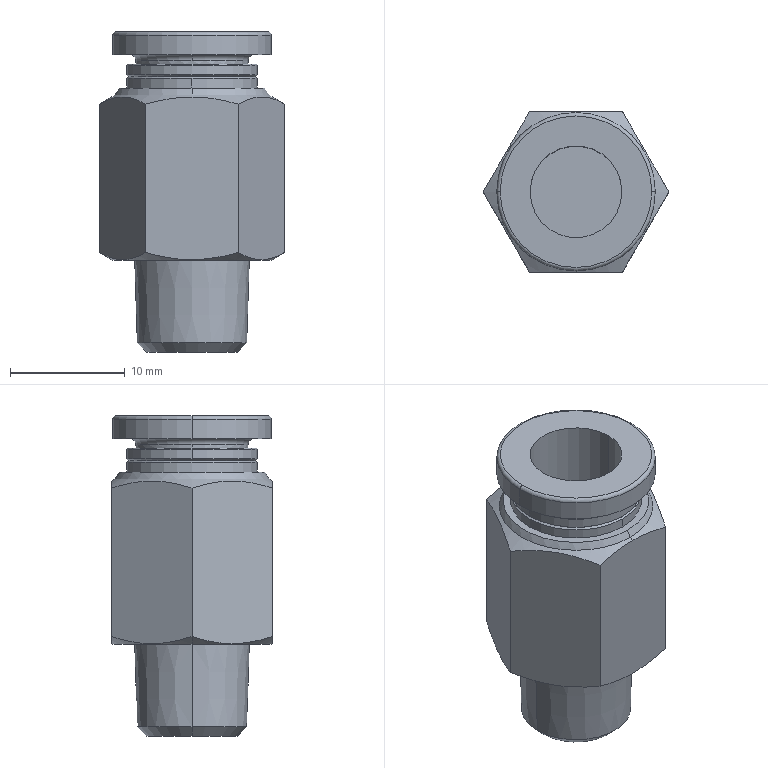Part | STEP file | PN_0022_default | 1 solid | 43 faces | box 16.166 x 14 x 27.9 mm | volume 2758 mm3 | cone 16 | plane 13 | cylinder 10 | torus 4 | commonest cylinder face diameters 11.4 x4 8 x2 9.8 x2 13.8 x2